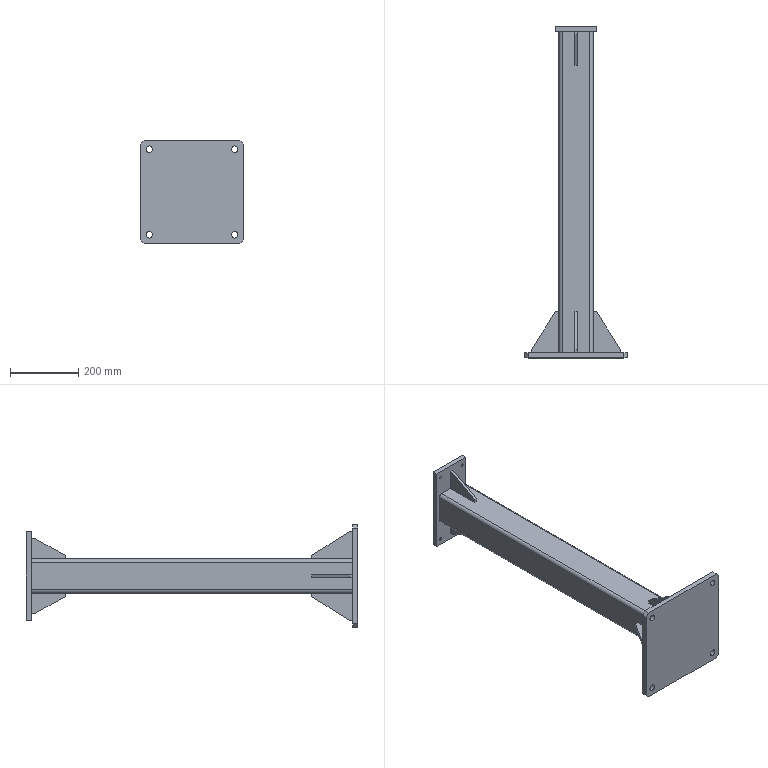Part | SolidWorks | features Gusset 12, HoleWzd 4, ICE 4, 3DProfileFeature 2, Chamfer 2, MirrorPattern 1, WeldMemberFeat 1, WeldmentFeature 1 | 9 solids | 104 faces | box 300 x 970 x 300 mm | volume 3763524 mm3 | plane 68 | cylinder 36 | commonest cylinder face diameters 5 x12 6.8 x8 19 x8 10 x4 20 x4